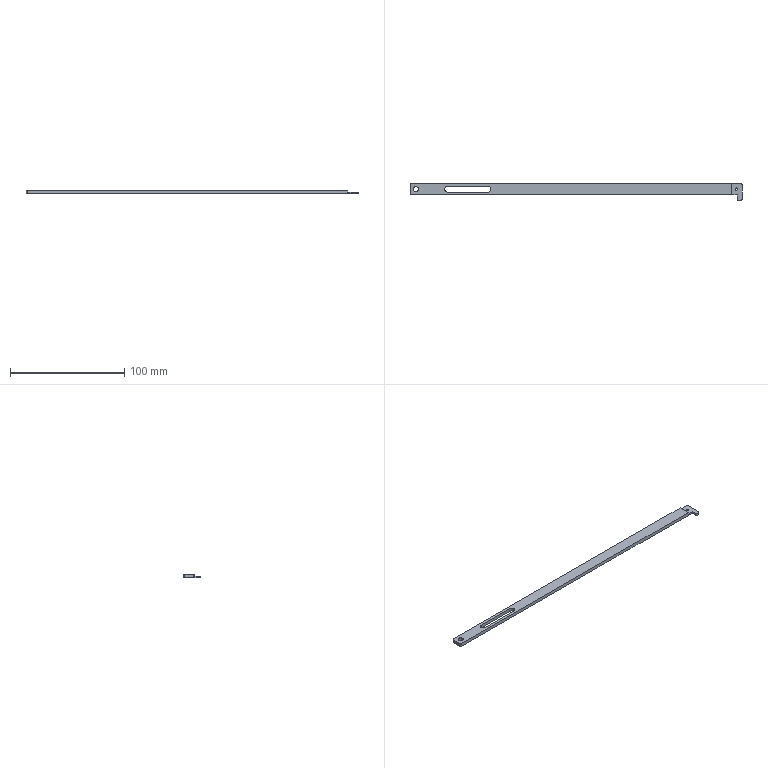Part | NX | features BREP 1 | 1 solid | 24 faces | box 290 x 15 x 3 mm | volume 7930 mm3 | plane 12 | cylinder 12 | commonest cylinder face diameters 2 x5 5.2 x3 2.05 x2 4.5 x2
STEP:
#1=CARTESIAN_POINT('',(-112.,-2.6,3.));
#2=VERTEX_POINT('',#1);
#3=CARTESIAN_POINT('',(-77.,-2.6,3.));
#4=VERTEX_POINT('',#3);
#5=CARTESIAN_POINT('',(-112.,-2.6,3.));
#6=DIRECTION('',(1.,0.,0.));
#7=VECTOR('',#6,1000.);
#8=LINE('',#5,#7);
#9=EDGE_CURVE('',#2,#4,#8,.T.);
#10=ORIENTED_EDGE('',*,*,#9,.T.);
#11=CARTESIAN_POINT('',(-77.,-2.6,0.));
#12=VERTEX_POINT('',#11);
#13=CARTESIAN_POINT('',(-77.,-2.6,0.));
#14=DIRECTION('',(0.,0.,1.));
#15=VECTOR('',#14,1000.);
#16=LINE('',#13,#15);
#17=EDGE_CURVE('',#12,#4,#16,.T.);
#18=ORIENTED_EDGE('',*,*,#17,.F.);
#19=CARTESIAN_POINT('',(-112.,-2.6,0.));
#20=VERTEX_POINT('',#19);
#21=CARTESIAN_POINT('',(-112.,-2.6,0.));
#22=DIRECTION('',(1.,0.,0.));
#23=VECTOR('',#22,1000.);
#24=LINE('',#21,#23);
#25=EDGE_CURVE('',#20,#12,#24,.T.);
#26=ORIENTED_EDGE('',*,*,#25,.F.);
#27=CARTESIAN_POINT('',(-112.,-2.6,0.));
#28=DIRECTION('',(0.,0.,1.));
#29=VECTOR('',#28,1000.);
#30=LINE('',#27,#29);
#31=EDGE_CURVE('',#20,#2,#30,.T.);
#32=ORIENTED_EDGE('',*,*,#31,.T.);
#33=EDGE_LOOP('',(#10,#18,#26,#32));
#34=FACE_BOUND('',#33,.T.);
#35=CARTESIAN_POINT('',(-112.,-2.6,0.));
#36=DIRECTION('',(0.,-1.,0.));
#37=DIRECTION('',(0.,0.,-1.));
#38=AXIS2_PLACEMENT_3D('',#35,#36,#37);
#39=PLANE('',#38);
#40=ADVANCED_FACE('',(#34),#39,.F.);
#41=CARTESIAN_POINT('',(-74.4,0.,0.));
#42=VERTEX_POINT('',#41);
#43=CARTESIAN_POINT('',(-74.4,0.,3.));
#44=VERTEX_POINT('',#43);
#45=CARTESIAN_POINT('',(-74.4,0.,0.));
#46=DIRECTION('',(0.,0.,1.));
#47=VECTOR('',#46,1000.);
#48=LINE('',#45,#47);
#49=EDGE_CURVE('',#42,#44,#48,.T.);
#50=ORIENTED_EDGE('',*,*,#49,.F.);
#51=CARTESIAN_POINT('',(-77.,0.,0.));
#52=DIRECTION('',(0.,0.,1.));
#53=DIRECTION('',(1.,0.,0.));
#54=AXIS2_PLACEMENT_3D('',#51,#52,#53);
#55=CIRCLE('',#54,2.6);
#56=EDGE_CURVE('',#12,#42,#55,.T.);
#57=ORIENTED_EDGE('',*,*,#56,.F.);
#58=ORIENTED_EDGE('',*,*,#17,.T.);
#59=CARTESIAN_POINT('',(-77.,0.,3.));
#60=DIRECTION('',(0.,0.,1.));
#61=DIRECTION('',(1.,0.,0.));
#62=AXIS2_PLACEMENT_3D('',#59,#60,#61);
#63=CIRCLE('',#62,2.6);
#64=EDGE_CURVE('',#4,#44,#63,.T.);
#65=ORIENTED_EDGE('',*,*,#64,.T.);
#66=EDGE_LOOP('',(#50,#57,#58,#65));
#67=FACE_BOUND('',#66,.T.);
#68=CARTESIAN_POINT('',(-77.,0.,0.));
#69=DIRECTION('',(0.,0.,1.));
#70=DIRECTION('',(1.,0.,0.));
#71=AXIS2_PLACEMENT_3D('',#68,#69,#70);
#72=CYLINDRICAL_SURFACE('',#71,2.6);
#73=ADVANCED_FACE('',(#67),#72,.F.);
#74=CARTESIAN_POINT('',(-77.,2.6,3.));
#75=VERTEX_POINT('',#74);
#76=CARTESIAN_POINT('',(-112.,2.6,3.));
#77=VERTEX_POINT('',#76);
#78=CARTESIAN_POINT('',(-112.,2.6,3.));
#79=DIRECTION('',(-1.,0.,0.));
#80=VECTOR('',#79,1000.);
#81=LINE('',#78,#80);
#82=EDGE_CURVE('',#75,#77,#81,.T.);
#83=ORIENTED_EDGE('',*,*,#82,.T.);
#84=CARTESIAN_POINT('',(-112.,2.6,0.));
#85=VERTEX_POINT('',#84);
#86=CARTESIAN_POINT('',(-112.,2.6,0.));
#87=DIRECTION('',(0.,0.,1.));
#88=VECTOR('',#87,1000.);
#89=LINE('',#86,#88);
#90=EDGE_CURVE('',#85,#77,#89,.T.);
#91=ORIENTED_EDGE('',*,*,#90,.F.);
#92=CARTESIAN_POINT('',(-77.,2.6,0.));
#93=VERTEX_POINT('',#92);
#94=CARTESIAN_POINT('',(-112.,2.6,0.));
#95=DIRECTION('',(-1.,0.,0.));
#96=VECTOR('',#95,1000.);
#97=LINE('',#94,#96);
#98=EDGE_CURVE('',#93,#85,#97,.T.);
#99=ORIENTED_EDGE('',*,*,#98,.F.);
#100=CARTESIAN_POINT('',(-77.,2.6,0.));
#101=DIRECTION('',(0.,0.,1.));
#102=VECTOR('',#101,1000.);
#103=LINE('',#100,#102);
#104=EDGE_CURVE('',#93,#75,#103,.T.);
#105=ORIENTED_EDGE('',*,*,#104,.T.);
#106=EDGE_LOOP('',(#83,#91,#99,#105));
#107=FACE_BOUND('',#106,.T.);
#108=CARTESIAN_POINT('',(-112.,2.6,0.));
#109=DIRECTION('',(0.,1.,0.));
#110=DIRECTION('',(0.,0.,1.));
#111=AXIS2_PLACEMENT_3D('',#108,#109,#110);
#112=PLANE('',#111);
#113=ADVANCED_FACE('',(#107),#112,.F.);
#114=CARTESIAN_POINT('',(-112.,0.,3.));
#115=DIRECTION('',(0.,0.,1.));
#116=DIRECTION('',(1.,0.,0.));
#117=AXIS2_PLACEMENT_3D('',#114,#115,#116);
#118=CIRCLE('',#117,2.6);
#119=EDGE_CURVE('',#77,#2,#118,.T.);
#120=ORIENTED_EDGE('',*,*,#119,.T.);
#121=ORIENTED_EDGE('',*,*,#31,.F.);
#122=CARTESIAN_POINT('',(-112.,0.,0.));
#123=DIRECTION('',(0.,0.,1.));
#124=DIRECTION('',(1.,0.,0.));
#125=AXIS2_PLACEMENT_3D('',#122,#123,#124);
#126=CIRCLE('',#125,2.6);
#127=EDGE_CURVE('',#85,#20,#126,.T.);
#128=ORIENTED_EDGE('',*,*,#127,.F.);
#129=ORIENTED_EDGE('',*,*,#90,.T.);
#130=EDGE_LOOP('',(#120,#121,#128,#129));
#131=FACE_BOUND('',#130,.T.);
#132=CARTESIAN_POINT('',(-112.,0.,0.));
#133=DIRECTION('',(0.,0.,1.));
#134=DIRECTION('',(1.,0.,0.));
#135=AXIS2_PLACEMENT_3D('',#132,#133,#134);
#136=CYLINDRICAL_SURFACE('',#135,2.6);
#137=ADVANCED_FACE('',(#131),#136,.F.);
#138=CARTESIAN_POINT('',(136.,-5.,1.5));
#139=VERTEX_POINT('',#138);
#140=CARTESIAN_POINT('',(141.,-5.,1.5));
#141=VERTEX_POINT('',#140);
#142=CARTESIAN_POINT('',(-145.,-5.,1.5));
#143=DIRECTION('',(1.,0.,0.));
#144=VECTOR('',#143,1000.);
#145=LINE('',#142,#144);
#146=EDGE_CURVE('',#139,#141,#145,.T.);
#147=ORIENTED_EDGE('',*,*,#146,.T.);
#148=CARTESIAN_POINT('',(141.,-9.,1.5));
#149=VERTEX_POINT('',#148);
#150=CARTESIAN_POINT('',(141.,-5.,1.5));
#151=DIRECTION('',(0.,1.,0.));
#152=VECTOR('',#151,1000.);
#153=LINE('',#150,#152);
#154=EDGE_CURVE('',#149,#141,#153,.T.);
#155=ORIENTED_EDGE('',*,*,#154,.F.);
#156=CARTESIAN_POINT('',(142.,-10.,1.5));
#157=VERTEX_POINT('',#156);
#158=CARTESIAN_POINT('',(142.,-9.,1.5));
#159=DIRECTION('',(0.,0.,-1.));
#160=DIRECTION('',(1.,0.,0.));
#161=AXIS2_PLACEMENT_3D('',#158,#159,#160);
#162=CIRCLE('',#161,1.);
#163=EDGE_CURVE('',#157,#149,#162,.T.);
#164=ORIENTED_EDGE('',*,*,#163,.F.);
#165=CARTESIAN_POINT('',(144.,-10.,1.5));
#166=VERTEX_POINT('',#165);
#167=CARTESIAN_POINT('',(145.,-10.,1.5));
#168=DIRECTION('',(1.,0.,0.));
#169=VECTOR('',#168,1000.);
#170=LINE('',#167,#169);
#171=EDGE_CURVE('',#157,#166,#170,.T.);
#172=ORIENTED_EDGE('',*,*,#171,.T.);
#173=CARTESIAN_POINT('',(145.,-9.,1.5));
#174=VERTEX_POINT('',#173);
#175=CARTESIAN_POINT('',(144.,-9.,1.5));
#176=DIRECTION('',(0.,0.,-1.));
#177=DIRECTION('',(1.,0.,0.));
#178=AXIS2_PLACEMENT_3D('',#175,#176,#177);
#179=CIRCLE('',#178,1.);
#180=EDGE_CURVE('',#174,#166,#179,.T.);
#181=ORIENTED_EDGE('',*,*,#180,.F.);
#182=CARTESIAN_POINT('',(145.,4.,1.5));
#183=VERTEX_POINT('',#182);
#184=CARTESIAN_POINT('',(145.,-10.,1.5));
#185=DIRECTION('',(0.,1.,0.));
#186=VECTOR('',#185,1000.);
#187=LINE('',#184,#186);
#188=EDGE_CURVE('',#174,#183,#187,.T.);
#189=ORIENTED_EDGE('',*,*,#188,.T.);
#190=CARTESIAN_POINT('',(144.,5.,1.5));
#191=VERTEX_POINT('',#190);
#192=CARTESIAN_POINT('',(144.,4.,1.5));
#193=DIRECTION('',(0.,0.,-1.));
#194=DIRECTION('',(1.,0.,0.));
#195=AXIS2_PLACEMENT_3D('',#192,#193,#194);
#196=CIRCLE('',#195,1.);
#197=EDGE_CURVE('',#191,#183,#196,.T.);
#198=ORIENTED_EDGE('',*,*,#197,.F.);
#199=CARTESIAN_POINT('',(136.,5.,1.5));
#200=VERTEX_POINT('',#199);
#201=CARTESIAN_POINT('',(145.,5.,1.5));
#202=DIRECTION('',(-1.,0.,0.));
#203=VECTOR('',#202,1000.);
#204=LINE('',#201,#203);
#205=EDGE_CURVE('',#191,#200,#204,.T.);
#206=ORIENTED_EDGE('',*,*,#205,.T.);
#207=CARTESIAN_POINT('',(136.,-10.,1.5));
#208=DIRECTION('',(0.,-1.,0.));
#209=VECTOR('',#208,1000.);
#210=LINE('',#207,#209);
#211=EDGE_CURVE('',#200,#139,#210,.T.);
#212=ORIENTED_EDGE('',*,*,#211,.T.);
#213=EDGE_LOOP('',(#147,#155,#164,#172,#181,#189,#198,#206,#212));
#214=FACE_BOUND('',#213,.T.);
#215=CARTESIAN_POINT('',(141.025,0.,1.5));
#216=VERTEX_POINT('',#215);
#217=CARTESIAN_POINT('',(138.975,0.,1.5));
#218=VERTEX_POINT('',#217);
#219=CARTESIAN_POINT('',(140.,0.,1.5));
#220=DIRECTION('',(0.,0.,-1.));
#221=DIRECTION('',(1.,0.,0.));
#222=AXIS2_PLACEMENT_3D('',#219,#220,#221);
#223=CIRCLE('',#222,1.025);
#224=EDGE_CURVE('',#216,#218,#223,.T.);
#225=ORIENTED_EDGE('',*,*,#224,.T.);
#226=CARTESIAN_POINT('',(140.,0.,1.5));
#227=DIRECTION('',(0.,0.,-1.));
#228=DIRECTION('',(1.,0.,0.));
#229=AXIS2_PLACEMENT_3D('',#226,#227,#228);
#230=CIRCLE('',#229,1.025);
#231=EDGE_CURVE('',#218,#216,#230,.T.);
#232=ORIENTED_EDGE('',*,*,#231,.T.);
#233=EDGE_LOOP('',(#225,#232));
#234=FACE_BOUND('',#233,.T.);
#235=CARTESIAN_POINT('',(0.,0.,1.5));
#236=DIRECTION('',(0.,0.,1.));
#237=DIRECTION('',(1.,0.,0.));
#238=AXIS2_PLACEMENT_3D('',#235,#236,#237);
#239=PLANE('',#238);
#240=ADVANCED_FACE('',(#214,#234),#239,.T.);
#241=ORIENTED_EDGE('',*,*,#211,.F.);
#242=CARTESIAN_POINT('',(136.,5.,3.));
#243=VERTEX_POINT('',#242);
#244=CARTESIAN_POINT('',(136.,5.,1.5));
#245=DIRECTION('',(0.,0.,1.));
#246=VECTOR('',#245,1000.);
#247=LINE('',#244,#246);
#248=EDGE_CURVE('',#200,#243,#247,.T.);
#249=ORIENTED_EDGE('',*,*,#248,.T.);
#250=CARTESIAN_POINT('',(136.,-5.,3.));
#251=VERTEX_POINT('',#250);
#252=CARTESIAN_POINT('',(136.,-10.,3.));
#253=DIRECTION('',(0.,-1.,0.));
#254=VECTOR('',#253,1000.);
#255=LINE('',#252,#254);
#256=EDGE_CURVE('',#243,#251,#255,.T.);
#257=ORIENTED_EDGE('',*,*,#256,.T.);
#258=CARTESIAN_POINT('',(136.,-5.,3.));
#259=DIRECTION('',(0.,0.,1.));
#260=VECTOR('',#259,1000.);
#261=LINE('',#258,#260);
#262=EDGE_CURVE('',#139,#251,#261,.T.);
#263=ORIENTED_EDGE('',*,*,#262,.F.);
#264=EDGE_LOOP('',(#241,#249,#257,#263));
#265=FACE_BOUND('',#264,.T.);
#266=CARTESIAN_POINT('',(136.,-10.,1.5));
#267=DIRECTION('',(-1.,0.,0.));
#268=DIRECTION('',(0.,0.,1.));
#269=AXIS2_PLACEMENT_3D('',#266,#267,#268);
#270=PLANE('',#269);
#271=ADVANCED_FACE('',(#265),#270,.F.);
#272=CARTESIAN_POINT('',(-145.,-4.,3.));
#273=VERTEX_POINT('',#272);
#274=CARTESIAN_POINT('',(-144.,-5.,3.));
#275=VERTEX_POINT('',#274);
#276=CARTESIAN_POINT('',(-144.,-4.,3.));
#277=DIRECTION('',(0.,0.,1.));
#278=DIRECTION('',(-1.,0.,0.));
#279=AXIS2_PLACEMENT_3D('',#276,#277,#278);
#280=CIRCLE('',#279,1.);
#281=EDGE_CURVE('',#273,#275,#280,.T.);
#282=ORIENTED_EDGE('',*,*,#281,.F.);
#283=CARTESIAN_POINT('',(-145.,-4.,0.));
#284=VERTEX_POINT('',#283);
#285=CARTESIAN_POINT('',(-145.,-4.,3.));
#286=DIRECTION('',(0.,0.,1.));
#287=VECTOR('',#286,1000.);
#288=LINE('',#285,#287);
#289=EDGE_CURVE('',#284,#273,#288,.T.);
#290=ORIENTED_EDGE('',*,*,#289,.F.);
#291=CARTESIAN_POINT('',(-144.,-5.,0.));
#292=VERTEX_POINT('',#291);
#293=CARTESIAN_POINT('',(-144.,-4.,0.));
#294=DIRECTION('',(0.,0.,-1.));
#295=DIRECTION('',(-1.,0.,0.));
#296=AXIS2_PLACEMENT_3D('',#293,#294,#295);
#297=CIRCLE('',#296,1.);
#298=EDGE_CURVE('',#292,#284,#297,.T.);
#299=ORIENTED_EDGE('',*,*,#298,.F.);
#300=CARTESIAN_POINT('',(-144.,-5.,3.));
#301=DIRECTION('',(0.,0.,-1.));
#302=VECTOR('',#301,1000.);
#303=LINE('',#300,#302);
#304=EDGE_CURVE('',#275,#292,#303,.T.);
#305=ORIENTED_EDGE('',*,*,#304,.F.);
#306=EDGE_LOOP('',(#282,#290,#299,#305));
#307=FACE_BOUND('',#306,.T.);
#308=CARTESIAN_POINT('',(-144.,-4.,3.));
#309=DIRECTION('',(0.,0.,-1.));
#310=DIRECTION('',(-1.,0.,0.));
#311=AXIS2_PLACEMENT_3D('',#308,#309,#310);
#312=CYLINDRICAL_SURFACE('',#311,1.);
#313=ADVANCED_FACE('',(#307),#312,.T.);
#314=CARTESIAN_POINT('',(-144.,5.,3.));
#315=VERTEX_POINT('',#314);
#316=CARTESIAN_POINT('',(-145.,4.,3.));
#317=VERTEX_POINT('',#316);
#318=CARTESIAN_POINT('',(-144.,4.,3.));
#319=DIRECTION('',(0.,0.,1.));
#320=DIRECTION('',(-1.,0.,0.));
#321=AXIS2_PLACEMENT_3D('',#318,#319,#320);
#322=CIRCLE('',#321,1.);
#323=EDGE_CURVE('',#315,#317,#322,.T.);
#324=ORIENTED_EDGE('',*,*,#323,.F.);
#325=CARTESIAN_POINT('',(-144.,5.,0.));
#326=VERTEX_POINT('',#325);
#327=CARTESIAN_POINT('',(-144.,5.,3.));
#328=DIRECTION('',(0.,0.,1.));
#329=VECTOR('',#328,1000.);
#330=LINE('',#327,#329);
#331=EDGE_CURVE('',#326,#315,#330,.T.);
#332=ORIENTED_EDGE('',*,*,#331,.F.);
#333=CARTESIAN_POINT('',(-145.,4.,0.));
#334=VERTEX_POINT('',#333);
#335=CARTESIAN_POINT('',(-144.,4.,0.));
#336=DIRECTION('',(0.,0.,-1.));
#337=DIRECTION('',(-1.,0.,0.));
#338=AXIS2_PLACEMENT_3D('',#335,#336,#337);
#339=CIRCLE('',#338,1.);
#340=EDGE_CURVE('',#334,#326,#339,.T.);
#341=ORIENTED_EDGE('',*,*,#340,.F.);
#342=CARTESIAN_POINT('',(-145.,4.,3.));
#343=DIRECTION('',(0.,0.,-1.));
#344=VECTOR('',#343,1000.);
#345=LINE('',#342,#344);
#346=EDGE_CURVE('',#317,#334,#345,.T.);
#347=ORIENTED_EDGE('',*,*,#346,.F.);
#348=EDGE_LOOP('',(#324,#332,#341,#347));
#349=FACE_BOUND('',#348,.T.);
#350=CARTESIAN_POINT('',(-144.,4.,3.));
#351=DIRECTION('',(0.,0.,-1.));
#352=DIRECTION('',(-1.,0.,0.));
#353=AXIS2_PLACEMENT_3D('',#350,#351,#352);
#354=CYLINDRICAL_SURFACE('',#353,1.);
#355=ADVANCED_FACE('',(#349),#354,.T.);
#356=CARTESIAN_POINT('',(-142.25,0.,3.));
#357=VERTEX_POINT('',#356);
#358=CARTESIAN_POINT('',(-142.25,0.,0.));
#359=VERTEX_POINT('',#358);
#360=CARTESIAN_POINT('',(-142.25,0.,3.));
#361=DIRECTION('',(0.,0.,1.));
#362=VECTOR('',#361,1000.);
#363=LINE('',#360,#362);
#364=EDGE_CURVE('',#357,#359,#363,.F.);
#365=ORIENTED_EDGE('',*,*,#364,.T.);
#366=CARTESIAN_POINT('',(-137.75,0.,0.));
#367=VERTEX_POINT('',#366);
#368=CARTESIAN_POINT('',(-140.,0.,0.));
#369=DIRECTION('',(0.,0.,1.));
#370=DIRECTION('',(1.,0.,0.));
#371=AXIS2_PLACEMENT_3D('',#368,#369,#370);
#372=CIRCLE('',#371,2.25);
#373=EDGE_CURVE('',#367,#359,#372,.T.);
#374=ORIENTED_EDGE('',*,*,#373,.F.);
#375=CARTESIAN_POINT('',(-137.75,0.,3.));
#376=VERTEX_POINT('',#375);
#377=CARTESIAN_POINT('',(-137.75,0.,3.));
#378=DIRECTION('',(0.,0.,1.));
#379=VECTOR('',#378,1000.);
#380=LINE('',#377,#379);
#381=EDGE_CURVE('',#376,#367,#380,.F.);
#382=ORIENTED_EDGE('',*,*,#381,.F.);
#383=CARTESIAN_POINT('',(-140.,0.,3.));
#384=DIRECTION('',(0.,0.,1.));
#385=DIRECTION('',(1.,0.,0.));
#386=AXIS2_PLACEMENT_3D('',#383,#384,#385);
#387=CIRCLE('',#386,2.25);
#388=EDGE_CURVE('',#376,#357,#387,.T.);
#389=ORIENTED_EDGE('',*,*,#388,.T.);
#390=EDGE_LOOP('',(#365,#374,#382,#389));
#391=FACE_BOUND('',#390,.T.);
#392=CARTESIAN_POINT('',(-140.,0.,3.));
#393=DIRECTION('',(0.,0.,1.));
#394=DIRECTION('',(1.,0.,0.));
#395=AXIS2_PLACEMENT_3D('',#392,#393,#394);
#396=CYLINDRICAL_SURFACE('',#395,2.25);
#397=ADVANCED_FACE('',(#391),#396,.F.);
#398=CARTESIAN_POINT('',(142.,-10.,0.));
#399=VERTEX_POINT('',#398);
#400=CARTESIAN_POINT('',(144.,-10.,0.));
#401=VERTEX_POINT('',#400);
#402=CARTESIAN_POINT('',(145.,-10.,0.));
#403=DIRECTION('',(1.,0.,0.));
#404=VECTOR('',#403,1000.);
#405=LINE('',#402,#404);
#406=EDGE_CURVE('',#399,#401,#405,.T.);
#407=ORIENTED_EDGE('',*,*,#406,.F.);
#408=CARTESIAN_POINT('',(141.,-9.,0.));
#409=VERTEX_POINT('',#408);
#410=CARTESIAN_POINT('',(142.,-9.,0.));
#411=DIRECTION('',(0.,0.,-1.));
#412=DIRECTION('',(-1.,0.,0.));
#413=AXIS2_PLACEMENT_3D('',#410,#411,#412);
#414=CIRCLE('',#413,1.);
#415=EDGE_CURVE('',#399,#409,#414,.T.);
#416=ORIENTED_EDGE('',*,*,#415,.T.);
#417=CARTESIAN_POINT('',(141.,-5.,0.));
#418=VERTEX_POINT('',#417);
#419=CARTESIAN_POINT('',(141.,-5.,0.));
#420=DIRECTION('',(0.,-1.,0.));
#421=VECTOR('',#420,1000.);
#422=LINE('',#419,#421);
#423=EDGE_CURVE('',#418,#409,#422,.T.);
#424=ORIENTED_EDGE('',*,*,#423,.F.);
#425=CARTESIAN_POINT('',(-145.,-5.,0.));
#426=DIRECTION('',(1.,0.,0.));
#427=VECTOR('',#426,1000.);
#428=LINE('',#425,#427);
#429=EDGE_CURVE('',#292,#418,#428,.T.);
#430=ORIENTED_EDGE('',*,*,#429,.F.);
#431=ORIENTED_EDGE('',*,*,#298,.T.);
#432=CARTESIAN_POINT('',(-145.,-5.,0.));
#433=DIRECTION('',(0.,-1.,0.));
#434=VECTOR('',#433,1000.);
#435=LINE('',#432,#434);
#436=EDGE_CURVE('',#334,#284,#435,.T.);
#437=ORIENTED_EDGE('',*,*,#436,.F.);
#438=ORIENTED_EDGE('',*,*,#340,.T.);
#439=CARTESIAN_POINT('',(144.,5.,0.));
#440=VERTEX_POINT('',#439);
#441=CARTESIAN_POINT('',(-145.,5.,0.));
#442=DIRECTION('',(-1.,0.,0.));
#443=VECTOR('',#442,1000.);
#444=LINE('',#441,#443);
#445=EDGE_CURVE('',#440,#326,#444,.T.);
#446=ORIENTED_EDGE('',*,*,#445,.F.);
#447=CARTESIAN_POINT('',(145.,4.,0.));
#448=VERTEX_POINT('',#447);
#449=CARTESIAN_POINT('',(144.,4.,0.));
#450=DIRECTION('',(0.,0.,-1.));
#451=DIRECTION('',(-1.,0.,0.));
#452=AXIS2_PLACEMENT_3D('',#449,#450,#451);
#453=CIRCLE('',#452,1.);
#454=EDGE_CURVE('',#440,#448,#453,.T.);
#455=ORIENTED_EDGE('',*,*,#454,.T.);
#456=CARTESIAN_POINT('',(145.,-9.,0.));
#457=VERTEX_POINT('',#456);
#458=CARTESIAN_POINT('',(145.,-5.,0.));
#459=DIRECTION('',(0.,1.,0.));
#460=VECTOR('',#459,1000.);
#461=LINE('',#458,#460);
#462=EDGE_CURVE('',#457,#448,#461,.T.);
#463=ORIENTED_EDGE('',*,*,#462,.F.);
#464=CARTESIAN_POINT('',(144.,-9.,0.));
#465=DIRECTION('',(0.,0.,-1.));
#466=DIRECTION('',(-1.,0.,0.));
#467=AXIS2_PLACEMENT_3D('',#464,#465,#466);
#468=CIRCLE('',#467,1.);
#469=EDGE_CURVE('',#457,#401,#468,.T.);
#470=ORIENTED_EDGE('',*,*,#469,.T.);
#471=EDGE_LOOP('',(#407,#416,#424,#430,#431,#437,#438,#446,#455,#463,#470));
#472=FACE_BOUND('',#471,.T.);
#473=ORIENTED_EDGE('',*,*,#373,.T.);
#474=CARTESIAN_POINT('',(-140.,0.,0.));
#475=DIRECTION('',(0.,0.,1.));
#476=DIRECTION('',(1.,0.,0.));
#477=AXIS2_PLACEMENT_3D('',#474,#475,#476);
#478=CIRCLE('',#477,2.25);
#479=EDGE_CURVE('',#359,#367,#478,.T.);
#480=ORIENTED_EDGE('',*,*,#479,.T.);
#481=EDGE_LOOP('',(#473,#480));
#482=FACE_BOUND('',#481,.T.);
#483=CARTESIAN_POINT('',(141.025,0.,0.));
#484=VERTEX_POINT('',#483);
#485=CARTESIAN_POINT('',(138.975,0.,0.));
#486=VERTEX_POINT('',#485);
#487=CARTESIAN_POINT('',(140.,0.,0.));
#488=DIRECTION('',(0.,0.,1.));
#489=DIRECTION('',(1.,0.,0.));
#490=AXIS2_PLACEMENT_3D('',#487,#488,#489);
#491=CIRCLE('',#490,1.025);
#492=EDGE_CURVE('',#484,#486,#491,.T.);
#493=ORIENTED_EDGE('',*,*,#492,.T.);
#494=CARTESIAN_POINT('',(140.,0.,0.));
#495=DIRECTION('',(0.,0.,1.));
#496=DIRECTION('',(1.,0.,0.));
#497=AXIS2_PLACEMENT_3D('',#494,#495,#496);
#498=CIRCLE('',#497,1.025);
#499=EDGE_CURVE('',#486,#484,#498,.T.);
#500=ORIENTED_EDGE('',*,*,#499,.T.);
#501=EDGE_LOOP('',(#493,#500));
#502=FACE_BOUND('',#501,.T.);
#503=ORIENTED_EDGE('',*,*,#127,.T.);
#504=ORIENTED_EDGE('',*,*,#25,.T.);
#505=ORIENTED_EDGE('',*,*,#56,.T.);
#506=CARTESIAN_POINT('',(-77.,0.,0.));
#507=DIRECTION('',(0.,0.,1.));
#508=DIRECTION('',(1.,0.,0.));
#509=AXIS2_PLACEMENT_3D('',#506,#507,#508);
#510=CIRCLE('',#509,2.6);
#511=EDGE_CURVE('',#42,#93,#510,.T.);
#512=ORIENTED_EDGE('',*,*,#511,.T.);
#513=ORIENTED_EDGE('',*,*,#98,.T.);
#514=EDGE_LOOP('',(#503,#504,#505,#512,#513));
#515=FACE_BOUND('',#514,.T.);
#516=CARTESIAN_POINT('',(0.,0.,0.));
#517=DIRECTION('',(0.,0.,-1.));
#518=DIRECTION('',(-1.,0.,0.));
#519=AXIS2_PLACEMENT_3D('',#516,#517,#518);
#520=PLANE('',#519);
#521=ADVANCED_FACE('',(#472,#482,#502,#515),#520,.T.);
#522=CARTESIAN_POINT('',(-145.,-5.,3.));
#523=DIRECTION('',(1.,0.,0.));
#524=VECTOR('',#523,1000.);
#525=LINE('',#522,#524);
#526=EDGE_CURVE('',#275,#251,#525,.T.);
#527=ORIENTED_EDGE('',*,*,#526,.T.);
#528=ORIENTED_EDGE('',*,*,#256,.F.);
#529=CARTESIAN_POINT('',(-145.,5.,3.));
#530=DIRECTION('',(-1.,0.,0.));
#531=VECTOR('',#530,1000.);
#532=LINE('',#529,#531);
#533=EDGE_CURVE('',#243,#315,#532,.T.);
#534=ORIENTED_EDGE('',*,*,#533,.T.);
#535=ORIENTED_EDGE('',*,*,#323,.T.);
#536=CARTESIAN_POINT('',(-145.,-5.,3.));
#537=DIRECTION('',(0.,-1.,0.));
#538=VECTOR('',#537,1000.);
#539=LINE('',#536,#538);
#540=EDGE_CURVE('',#317,#273,#539,.T.);
#541=ORIENTED_EDGE('',*,*,#540,.T.);
#542=ORIENTED_EDGE('',*,*,#281,.T.);
#543=EDGE_LOOP('',(#527,#528,#534,#535,#541,#542));
#544=FACE_BOUND('',#543,.T.);
#545=ORIENTED_EDGE('',*,*,#388,.F.);
#546=CARTESIAN_POINT('',(-140.,0.,3.));
#547=DIRECTION('',(0.,0.,1.));
#548=DIRECTION('',(1.,0.,0.));
#549=AXIS2_PLACEMENT_3D('',#546,#547,#548);
#550=CIRCLE('',#549,2.25);
#551=EDGE_CURVE('',#357,#376,#550,.T.);
#552=ORIENTED_EDGE('',*,*,#551,.F.);
#553=EDGE_LOOP('',(#545,#552));
#554=FACE_BOUND('',#553,.T.);
#555=ORIENTED_EDGE('',*,*,#9,.F.);
#556=ORIENTED_EDGE('',*,*,#119,.F.);
#557=ORIENTED_EDGE('',*,*,#82,.F.);
#558=CARTESIAN_POINT('',(-77.,0.,3.));
#559=DIRECTION('',(0.,0.,1.));
#560=DIRECTION('',(1.,0.,0.));
#561=AXIS2_PLACEMENT_3D('',#558,#559,#560);
#562=CIRCLE('',#561,2.6);
#563=EDGE_CURVE('',#44,#75,#562,.T.);
#564=ORIENTED_EDGE('',*,*,#563,.F.);
#565=ORIENTED_EDGE('',*,*,#64,.F.);
#566=EDGE_LOOP('',(#555,#556,#557,#564,#565));
#567=FACE_BOUND('',#566,.T.);
#568=CARTESIAN_POINT('',(0.,0.,3.));
#569=DIRECTION('',(0.,0.,-1.));
#570=DIRECTION('',(-1.,0.,0.));
#571=AXIS2_PLACEMENT_3D('',#568,#569,#570);
#572=PLANE('',#571);
#573=ADVANCED_FACE('',(#544,#554,#567),#572,.F.);
#574=ORIENTED_EDGE('',*,*,#146,.F.);
#575=ORIENTED_EDGE('',*,*,#262,.T.);
#576=ORIENTED_EDGE('',*,*,#526,.F.);
#577=ORIENTED_EDGE('',*,*,#304,.T.);
#578=ORIENTED_EDGE('',*,*,#429,.T.);
#579=CARTESIAN_POINT('',(141.,-5.,-6.403));
#580=DIRECTION('',(0.,0.,1.));
#581=VECTOR('',#580,1000.);
#582=LINE('',#579,#581);
#583=EDGE_CURVE('',#418,#141,#582,.T.);
#584=ORIENTED_EDGE('',*,*,#583,.T.);
#585=EDGE_LOOP('',(#574,#575,#576,#577,#578,#584));
#586=FACE_BOUND('',#585,.T.);
#587=CARTESIAN_POINT('',(-145.,-5.,3.));
#588=DIRECTION('',(0.,1.,0.));
#589=DIRECTION('',(0.,0.,1.));
#590=AXIS2_PLACEMENT_3D('',#587,#588,#589);
#591=PLANE('',#590);
#592=ADVANCED_FACE('',(#586),#591,.F.);
#593=ORIENTED_EDGE('',*,*,#540,.F.);
#594=ORIENTED_EDGE('',*,*,#346,.T.);
#595=ORIENTED_EDGE('',*,*,#436,.T.);
#596=ORIENTED_EDGE('',*,*,#289,.T.);
#597=EDGE_LOOP('',(#593,#594,#595,#596));
#598=FACE_BOUND('',#597,.T.);
#599=CARTESIAN_POINT('',(-145.,-5.,3.));
#600=DIRECTION('',(1.,0.,0.));
#601=DIRECTION('',(0.,0.,-1.));
#602=AXIS2_PLACEMENT_3D('',#599,#600,#601);
#603=PLANE('',#602);
#604=ADVANCED_FACE('',(#598),#603,.F.);
#605=ORIENTED_EDGE('',*,*,#533,.F.);
#606=ORIENTED_EDGE('',*,*,#248,.F.);
#607=ORIENTED_EDGE('',*,*,#205,.F.);
#608=CARTESIAN_POINT('',(144.,5.,3.));
#609=DIRECTION('',(0.,0.,-1.));
#610=VECTOR('',#609,1000.);
#611=LINE('',#608,#610);
#612=EDGE_CURVE('',#191,#440,#611,.T.);
#613=ORIENTED_EDGE('',*,*,#612,.T.);
#614=ORIENTED_EDGE('',*,*,#445,.T.);
#615=ORIENTED_EDGE('',*,*,#331,.T.);
#616=EDGE_LOOP('',(#605,#606,#607,#613,#614,#615));
#617=FACE_BOUND('',#616,.T.);
#618=CARTESIAN_POINT('',(-145.,5.,3.));
#619=DIRECTION('',(0.,-1.,0.));
#620=DIRECTION('',(0.,0.,-1.));
#621=AXIS2_PLACEMENT_3D('',#618,#619,#620);
#622=PLANE('',#621);
#623=ADVANCED_FACE('',(#617),#622,.F.);
#624=CARTESIAN_POINT('',(138.975,0.,3.));
#625=DIRECTION('',(0.,0.,1.));
#626=VECTOR('',#625,1000.);
#627=LINE('',#624,#626);
#628=EDGE_CURVE('',#218,#486,#627,.F.);
#629=ORIENTED_EDGE('',*,*,#628,.T.);
#630=ORIENTED_EDGE('',*,*,#492,.F.);
#631=CARTESIAN_POINT('',(141.025,0.,3.));
#632=DIRECTION('',(0.,0.,1.));
#633=VECTOR('',#632,1000.);
#634=LINE('',#631,#633);
#635=EDGE_CURVE('',#216,#484,#634,.F.);
#636=ORIENTED_EDGE('',*,*,#635,.F.);
#637=ORIENTED_EDGE('',*,*,#231,.F.);
#638=EDGE_LOOP('',(#629,#630,#636,#637));
#639=FACE_BOUND('',#638,.T.);
#640=CARTESIAN_POINT('',(140.,0.,3.));
#641=DIRECTION('',(0.,0.,1.));
#642=DIRECTION('',(1.,0.,0.));
#643=AXIS2_PLACEMENT_3D('',#640,#641,#642);
#644=CYLINDRICAL_SURFACE('',#643,1.025);
#645=ADVANCED_FACE('',(#639),#644,.F.);
#646=CARTESIAN_POINT('',(145.,-9.,0.));
#647=DIRECTION('',(0.,0.,-1.));
#648=VECTOR('',#647,1000.);
#649=LINE('',#646,#648);
#650=EDGE_CURVE('',#174,#457,#649,.T.);
#651=ORIENTED_EDGE('',*,*,#650,.F.);
#652=ORIENTED_EDGE('',*,*,#180,.T.);
#653=CARTESIAN_POINT('',(144.,-10.,3.));
#654=DIRECTION('',(0.,0.,1.));
#655=VECTOR('',#654,1000.);
#656=LINE('',#653,#655);
#657=EDGE_CURVE('',#401,#166,#656,.T.);
#658=ORIENTED_EDGE('',*,*,#657,.F.);
#659=ORIENTED_EDGE('',*,*,#469,.F.);
#660=EDGE_LOOP('',(#651,#652,#658,#659));
#661=FACE_BOUND('',#660,.T.);
#662=CARTESIAN_POINT('',(144.,-9.,-6.403));
#663=DIRECTION('',(0.,0.,-1.));
#664=DIRECTION('',(-1.,0.,0.));
#665=AXIS2_PLACEMENT_3D('',#662,#663,#664);
#666=CYLINDRICAL_SURFACE('',#665,1.);
#667=ADVANCED_FACE('',(#661),#666,.T.);
#668=ORIENTED_EDGE('',*,*,#612,.F.);
#669=ORIENTED_EDGE('',*,*,#197,.T.);
#670=CARTESIAN_POINT('',(145.,4.,3.));
#671=DIRECTION('',(0.,0.,1.));
#672=VECTOR('',#671,1000.);
#673=LINE('',#670,#672);
#674=EDGE_CURVE('',#448,#183,#673,.T.);
#675=ORIENTED_EDGE('',*,*,#674,.F.);
#676=ORIENTED_EDGE('',*,*,#454,.F.);
#677=EDGE_LOOP('',(#668,#669,#675,#676));
#678=FACE_BOUND('',#677,.T.);
#679=CARTESIAN_POINT('',(144.,4.,3.));
#680=DIRECTION('',(0.,0.,-1.));
#681=DIRECTION('',(-1.,0.,0.));
#682=AXIS2_PLACEMENT_3D('',#679,#680,#681);
#683=CYLINDRICAL_SURFACE('',#682,1.);
#684=ADVANCED_FACE('',(#678),#683,.T.);
#685=CARTESIAN_POINT('',(142.,-10.,-6.403));
#686=DIRECTION('',(0.,0.,-1.));
#687=VECTOR('',#686,1000.);
#688=LINE('',#685,#687);
#689=EDGE_CURVE('',#157,#399,#688,.T.);
#690=ORIENTED_EDGE('',*,*,#689,.F.);
#691=ORIENTED_EDGE('',*,*,#163,.T.);
#692=CARTESIAN_POINT('',(141.,-9.,-6.403));
#693=DIRECTION('',(0.,0.,1.));
#694=VECTOR('',#693,1000.);
#695=LINE('',#692,#694);
#696=EDGE_CURVE('',#409,#149,#695,.T.);
#697=ORIENTED_EDGE('',*,*,#696,.F.);
#698=ORIENTED_EDGE('',*,*,#415,.F.);
#699=EDGE_LOOP('',(#690,#691,#697,#698));
#700=FACE_BOUND('',#699,.T.);
#701=CARTESIAN_POINT('',(142.,-9.,-6.403));
#702=DIRECTION('',(0.,0.,1.));
#703=DIRECTION('',(1.,0.,0.));
#704=AXIS2_PLACEMENT_3D('',#701,#702,#703);
#705=CYLINDRICAL_SURFACE('',#704,1.);
#706=ADVANCED_FACE('',(#700),#705,.T.);
#707=ORIENTED_EDGE('',*,*,#657,.T.);
#708=ORIENTED_EDGE('',*,*,#171,.F.);
#709=ORIENTED_EDGE('',*,*,#689,.T.);
#710=ORIENTED_EDGE('',*,*,#406,.T.);
#711=EDGE_LOOP('',(#707,#708,#709,#710));
#712=FACE_BOUND('',#711,.T.);
#713=CARTESIAN_POINT('',(145.,-10.,-6.403));
#714=DIRECTION('',(0.,-1.,0.));
#715=DIRECTION('',(1.,0.,0.));
#716=AXIS2_PLACEMENT_3D('',#713,#714,#715);
#717=PLANE('',#716);
#718=ADVANCED_FACE('',(#712),#717,.T.);
#719=ORIENTED_EDGE('',*,*,#696,.T.);
#720=ORIENTED_EDGE('',*,*,#154,.T.);
#721=ORIENTED_EDGE('',*,*,#583,.F.);
#722=ORIENTED_EDGE('',*,*,#423,.T.);
#723=EDGE_LOOP('',(#719,#720,#721,#722));
#724=FACE_BOUND('',#723,.T.);
#725=CARTESIAN_POINT('',(141.,-5.,-6.403));
#726=DIRECTION('',(-1.,0.,0.));
#727=DIRECTION('',(0.,0.,1.));
#728=AXIS2_PLACEMENT_3D('',#725,#726,#727);
#729=PLANE('',#728);
#730=ADVANCED_FACE('',(#724),#729,.T.);
#731=ORIENTED_EDGE('',*,*,#188,.F.);
#732=ORIENTED_EDGE('',*,*,#650,.T.);
#733=ORIENTED_EDGE('',*,*,#462,.T.);
#734=ORIENTED_EDGE('',*,*,#674,.T.);
#735=EDGE_LOOP('',(#731,#732,#733,#734));
#736=FACE_BOUND('',#735,.T.);
#737=CARTESIAN_POINT('',(145.,-5.,3.));
#738=DIRECTION('',(-1.,0.,0.));
#739=DIRECTION('',(0.,0.,1.));
#740=AXIS2_PLACEMENT_3D('',#737,#738,#739);
#741=PLANE('',#740);
#742=ADVANCED_FACE('',(#736),#741,.F.);
#743=ORIENTED_EDGE('',*,*,#499,.F.);
#744=ORIENTED_EDGE('',*,*,#628,.F.);
#745=ORIENTED_EDGE('',*,*,#224,.F.);
#746=ORIENTED_EDGE('',*,*,#635,.T.);
#747=EDGE_LOOP('',(#743,#744,#745,#746));
#748=FACE_BOUND('',#747,.T.);
#749=CARTESIAN_POINT('',(140.,0.,3.));
#750=DIRECTION('',(0.,0.,1.));
#751=DIRECTION('',(1.,0.,0.));
#752=AXIS2_PLACEMENT_3D('',#749,#750,#751);
#753=CYLINDRICAL_SURFACE('',#752,1.025);
#754=ADVANCED_FACE('',(#748),#753,.F.);
#755=ORIENTED_EDGE('',*,*,#479,.F.);
#756=ORIENTED_EDGE('',*,*,#364,.F.);
#757=ORIENTED_EDGE('',*,*,#551,.T.);
#758=ORIENTED_EDGE('',*,*,#381,.T.);
#759=EDGE_LOOP('',(#755,#756,#757,#758));
#760=FACE_BOUND('',#759,.T.);
#761=CARTESIAN_POINT('',(-140.,0.,3.));
#762=DIRECTION('',(0.,0.,1.));
#763=DIRECTION('',(1.,0.,0.));
#764=AXIS2_PLACEMENT_3D('',#761,#762,#763);
#765=CYLINDRICAL_SURFACE('',#764,2.25);
#766=ADVANCED_FACE('',(#760),#765,.F.);
#767=ORIENTED_EDGE('',*,*,#511,.F.);
#768=ORIENTED_EDGE('',*,*,#49,.T.);
#769=ORIENTED_EDGE('',*,*,#563,.T.);
#770=ORIENTED_EDGE('',*,*,#104,.F.);
#771=EDGE_LOOP('',(#767,#768,#769,#770));
#772=FACE_BOUND('',#771,.T.);
#773=CARTESIAN_POINT('',(-77.,0.,0.));
#774=DIRECTION('',(0.,0.,1.));
#775=DIRECTION('',(1.,0.,0.));
#776=AXIS2_PLACEMENT_3D('',#773,#774,#775);
#777=CYLINDRICAL_SURFACE('',#776,2.6);
#778=ADVANCED_FACE('',(#772),#777,.F.);
#779=CLOSED_SHELL('',(#40,#73,#113,#137,#240,#271,#313,#355,#397,#521,#573,#592,#604,#623,#645,#667,#684,#706,#718,#730,#742,#754,#766,#778));
#780=MANIFOLD_SOLID_BREP('',#779);
#781=(LENGTH_UNIT()NAMED_UNIT(*)SI_UNIT(.MILLI.,.METRE.));
#782=UNCERTAINTY_MEASURE_WITH_UNIT(LENGTH_MEASURE(0.00001),#781,'','');
#783=(NAMED_UNIT(*)PLANE_ANGLE_UNIT()SI_UNIT($,.RADIAN.));
#784=(NAMED_UNIT(*)SI_UNIT($,.STERADIAN.)SOLID_ANGLE_UNIT());
#785=(GEOMETRIC_REPRESENTATION_CONTEXT(3)GLOBAL_UNCERTAINTY_ASSIGNED_CONTEXT((#782))GLOBAL_UNIT_ASSIGNED_CONTEXT((#781,#783,#784))REPRESENTATION_CONTEXT('',''));
#786=ADVANCED_BREP_SHAPE_REPRESENTATION('',(#780),#785);